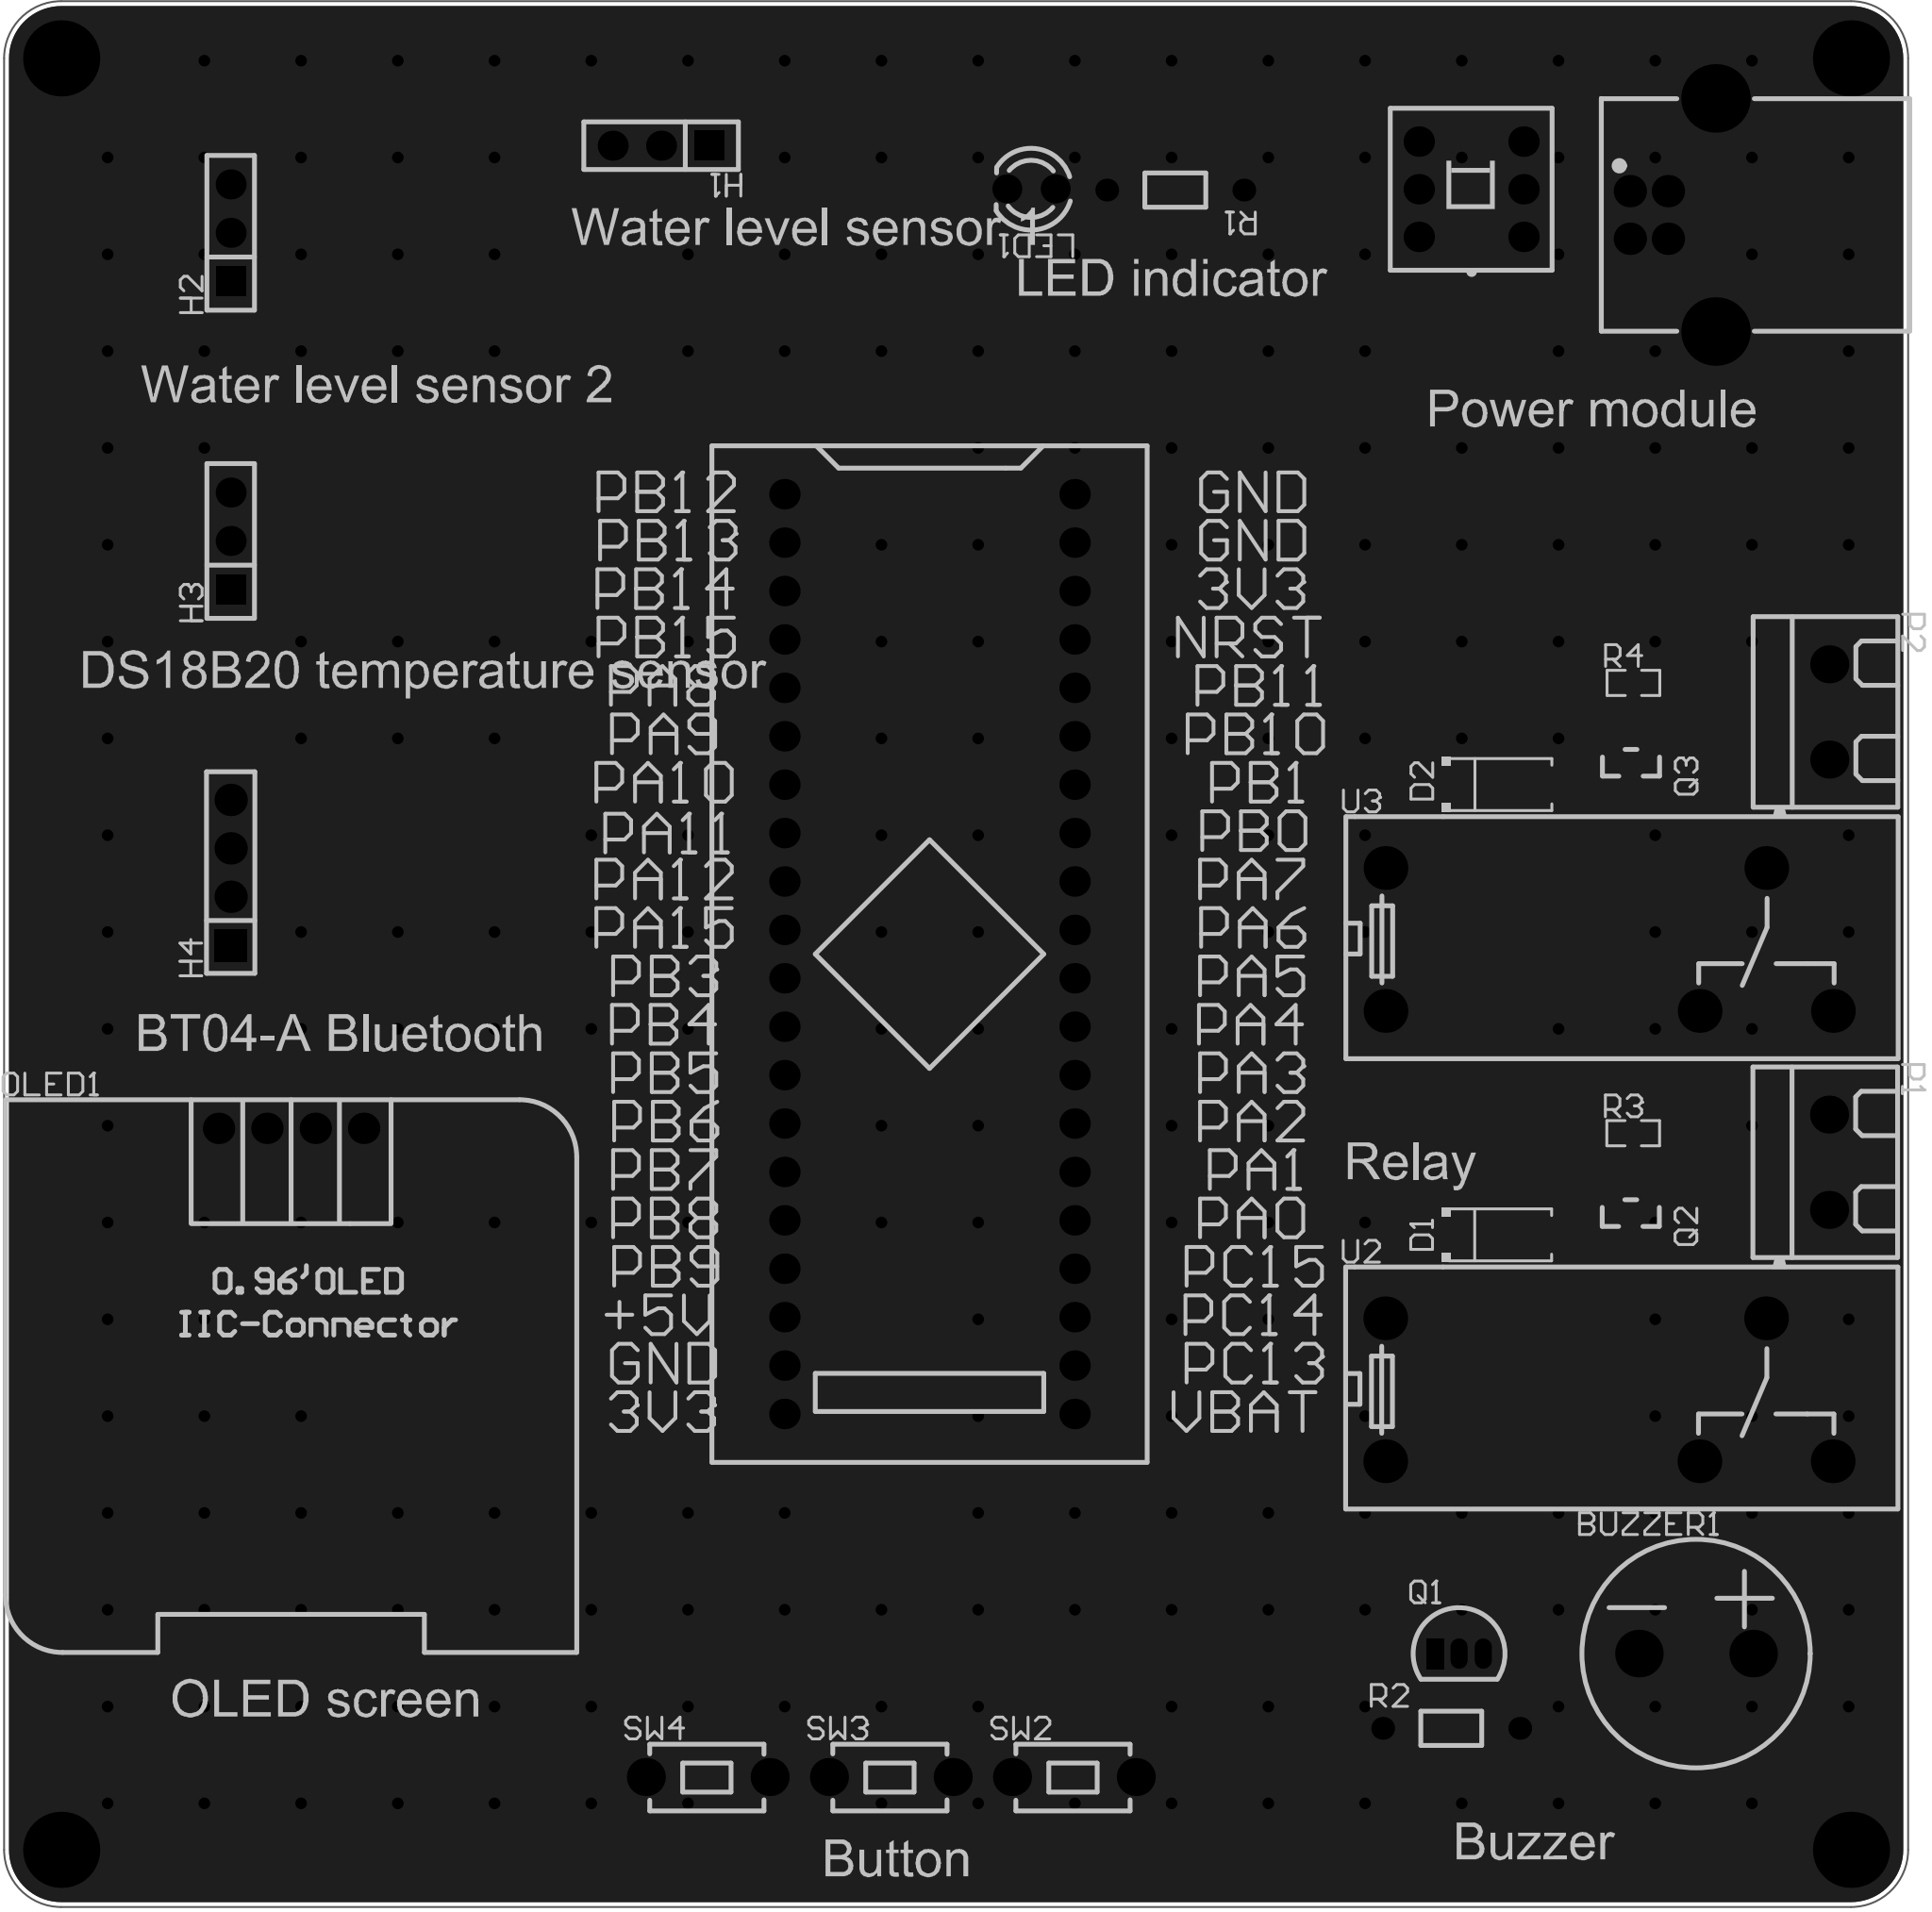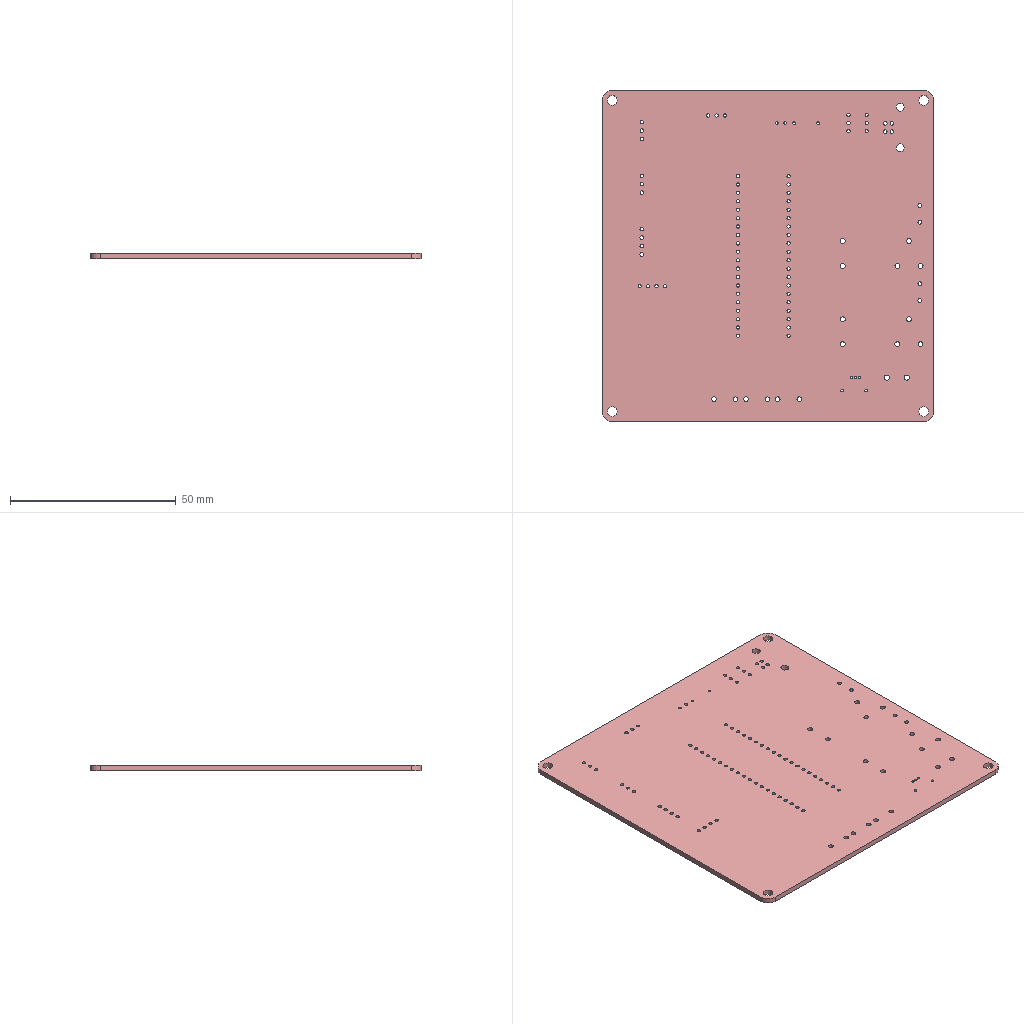Circuit board layout | Altium Designer | box 100 x 100 x 1.6 mm
Layer stack:
# Altium Designer layer stack of  (unit mm; dielectric type: 0 none, 1 core, 2 prepreg, 3 surface material)
index,name,kind,layer,copper_thickness_mm,dielectric_type,dielectric_thickness_mm,dielectric_material,dielectric_constant
0,Top Paste Mask Layer,other,,,,,,
1,Top Silkscreen Layer,other,,,,,,
2,Top Solder Mask Layer,dielectric,,,3,0.01,,3.3
3,Top Layer,copper,Top Layer,0.035,,,,
4,Dielectric1,dielectric,,,3,1.51,FR4,4.5
5,Bottom Layer,copper,Bottom Layer,0.035,,,,
6,Bottom Solder Mask Layer,dielectric,,,3,0.01,,3.3
7,Bottom Silkscreen Layer,other,,,,,,
8,Bottom Paste Mask Layer,other,,,,,,
# drill layer pairs: low layer,high layer
drill_pair,Top Layer,Bottom Layer
Part placement:
Designator,Comment,Layer,Footprint,Center-X(mm),Center-Y(mm),Rotation
U1,STM32F103C8T6-Card,TopLayer,CONN-TH_L53.3-W22.9_STM32F103C8T6-CARD,129.159,128.905,270
KEY1,Non-self-locking switch 8.5×8.5 silent,TopLayer,SW-TH_6P-L8.5-W8.5-P2.54,157.607,169.037,90
USB1,,TopLayer,USB__Type-B,168.191,167.688,90
BUZZER1,buzzer,TopLayer,BUZ-TH_BD12.0-P6.00-D0.9-RD,169.418,92.202,0
D1,,TopLayer,SMA_1N4007,159.131,114.173,0
D2,,TopLayer,SMA_1N4007,159.143,137.801,0
H1,,TopLayer,HDR-TH_3P-P2.54-V-F,115.062,171.323,180
H2,,TopLayer,HDR-TH_3P-P2.54-V-F,92.456,166.751,90
H3,,TopLayer,HDR-TH_3P-P2.54-V-F,92.456,150.582,90
H4,,TopLayer,HDR-TH_4P-P2.54-V-F,92.456,133.184,90
LED1,,TopLayer,LED_TH-3mm,134.49,169.056,180
OLED1,,TopLayer,0.96OLED_4P,95.631,119.761,0
P1,KF301-2P terminal block,TopLayer,CONN-TH_XY301V-A-5.0-2P,176.403,117.983,270
P2,KF301-2P terminal block,TopLayer,CONN-TH_XY301V-A-5.0-2P,176.415,141.611,270
Q1,,TopLayer,S8050_TO_92,156.972,92.202,0
Q2,,TopLayer,S8050_SOT-23,165.989,115.316,90
Q3,,TopLayer,S8050_SOT-23,166.001,138.944,90
R1,220,TopLayer,Res_1/8W,142.068,168.993,180
R2,10kΩ,TopLayer,Res_1/8W,156.561,88.282,0
R3,1K,TopLayer,R0603,166.116,119.507,0
R4,1K,TopLayer,R0603,166.128,143.135,0
SW2,,TopLayer,Key_TH_3.5x6x4.3,136.743,85.725,0
SW3,,TopLayer,Key_TH_3.5x6x4.3,127.128,85.725,0
SW4,,TopLayer,Key_TH_3.5x6x4.3,117.513,85.725,0
U2,SSKD6132,TopLayer,RELAY-TH_G2R-1,164.846,106.045,0
U3,SSKD6132,TopLayer,RELAY-TH_G2R-1,164.858,129.673,0
Pad and via stacks:
# Altium Designer via and pad stacks of  (unit mm). Each distinct definition once, with the count of objects using it.
# via: kind,start_layer,end_layer,hole_mm,diameter_mm,mode(0 simple;1 top-mid-bottom;2 full stack),diameter_per_layer,count,example_net
# pad: kind,layer,hole_mm,hole_type(0 round;1 square;2 slot),plating,top_size,top_shape(1 round;2 rect;3 octagon;9 rounded rect),mid_size,bottom_size,mode,footprint,size_per_layer,count,example
pad,Multi-Layer,3,0,plated,4x4,1,4x4,4x4,0,,,4,1
pad,Multi-Layer,1,0,plated,1.6x1.6,1,1.6x1.6,1.6x1.6,0,CONN-TH_L53.3-W22.9_STM32F103C8T6-CARD,,40,U1.1
pad,Multi-Layer,1,0,plated,1.6x1.6,1,1.6x1.6,1.6x1.6,0,SW-TH_6P-L8.5-W8.5-P2.54,,6,KEY1.4
pad,Multi-Layer,1.1,0,plated,1.7x1.7,1,1.7x1.7,1.7x1.7,0,USB_ Type-B,,4,USB1.3
pad,Multi-Layer,2.4,0,plated,3.6x3.6,1,3.6x3.6,3.6x3.6,0,USB_ Type-B,,2,USB1.5
pad,Multi-Layer,1.5,0,plated,2.5x2.5,1,2.5x2.5,2.5x2.5,0,BUZ-TH_BD12.0-P6.00-D0.9-RD,,2,BUZZER1.1
pad,Multi-Layer,1.02,0,plated,1.575x1.575,1,1.575x1.575,1.575x1.575,0,HDR-TH_3P-P2.54-V-F,,6,H1.3
pad,Multi-Layer,1.02,0,plated,1.575x1.575,2,1.575x1.575,1.575x1.575,0,HDR-TH_3P-P2.54-V-F,,3,H1.1
pad,Multi-Layer,1.1,0,plated,1.7x1.7,2,1.7x1.7,1.7x1.7,0,HDR-TH_4P-P2.54-V-F,,1,H4.1
pad,Multi-Layer,1.1,0,plated,1.7x1.7,1,1.7x1.7,1.7x1.7,0,HDR-TH_4P-P2.54-V-F,,3,H4.2
pad,Multi-Layer,0.9144,0,plated,1.524x1.524,1,1.524x1.524,1.524x1.524,0,LED_TH-3mm,,2,LED1.1
pad,Multi-Layer,1,0,plated,1.65x1.65,1,1.65x1.65,1.65x1.65,0,0.96OLED_4P,,4,OLED1.4
pad,Multi-Layer,1.2,0,plated,2x2,1,2x2,2x2,0,CONN-TH_XY301V-A-5.0-2P,,4,P1.1
pad,Multi-Layer,0.701,0,plated,0.8992x1.6,2,0.8992x1.6,0.8992x1.6,0,S8050_TO_92,,1,Q1.1
pad,Multi-Layer,0.701,0,plated,0.8992x1.6,1,0.8992x1.6,0.8992x1.6,0,S8050_TO_92,,2,Q1.2
pad,Multi-Layer,0.8001,0,plated,1.199x1.199,1,1.199x1.199,1.199x1.199,0,Res_1/8W,,4,R1.1
pad,Multi-Layer,1.399,0,plated,1.999x1.999,1,1.999x1.999,1.999x1.999,0,Key_TH_3.5x6x4.3,,6,SW2.A
pad,Multi-Layer,1.5,0,plated,2.3x2.3,1,2.3x2.3,2.3x2.3,0,RELAY-TH_G2R-1,,10,U2.3
pad,Top Layer,0,0,plated,2.046x1.62,2,2.046x1.62,2.046x1.62,0,SMA_1N4007,,4,D1.2
pad,Top Layer,0,0,plated,1x0.8,2,1x0.8,1x0.8,0,S8050_SOT-23,,6,Q2.2
pad,Top Layer,0,0,plated,0.8065x0.864,2,0.8065x0.864,0.8065x0.864,0,R0603,,4,R3.2
via,Top Layer,Bottom Layer,0.3048,0.61,0,,256,GND
Copper pours:
name,layer,net,type(0 solid;1 hatched;2 none)
Bottom Layer-GND,Bottom Layer,GND,0
Top Layer-GND,Top Layer,GND,0
Design rules, without the lines most boards share:
# Altium Designer design rules of  (exported by Altium Designer, unit mm)
# columns: name | kind | enabled | priority | scope1 | scope2 | descriptor | typed fields (field=value)
copperThickness1oz_2 | 2 | enabled | 2 | All | All | Width Constraint (Min=5mil) (Max=100mil) (Preferred=30mil) (All) |
viaSize | 11 | enabled | 1 | All | All | Routing Via (MinHoleWidth=11.811mil) (MaxHoleWidth=248.032mil) (PreferredHoleWidth=12.008mil) (MinWidth=19.685mil) (MaxWidth=393.701mil) (PreferedWidth=24.016mil) (All) | via_min_hole=0.3 via_max_hole=6.3 via_preferred_diameter=0.61 via_preferred_hole=0.305
solderMaskExpansion | 13 | enabled | 2 | All | All | Solder Mask Expansion (Expansion =2.008mil) (All) | expansion=0.051